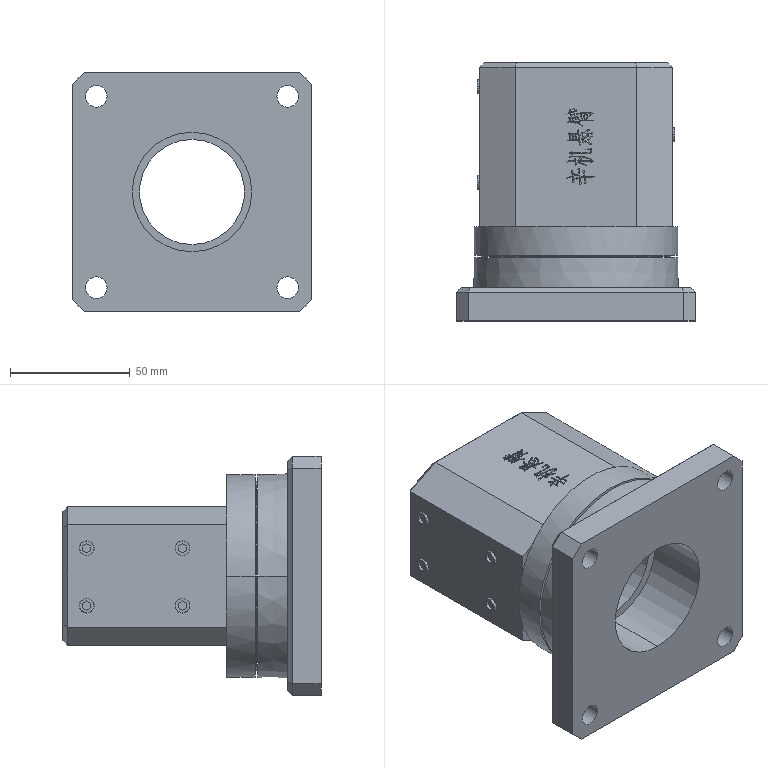Part | SolidWorks | 8 solids | 592 faces | box 100 x 108 x 100 mm | volume 341728 mm3 | plane 393 | spline 137 | cylinder 48 | cone 14 | commonest cylinder face diameters 6 x12 6.2 x12 9 x8 14 x8 44 x2 50 x2